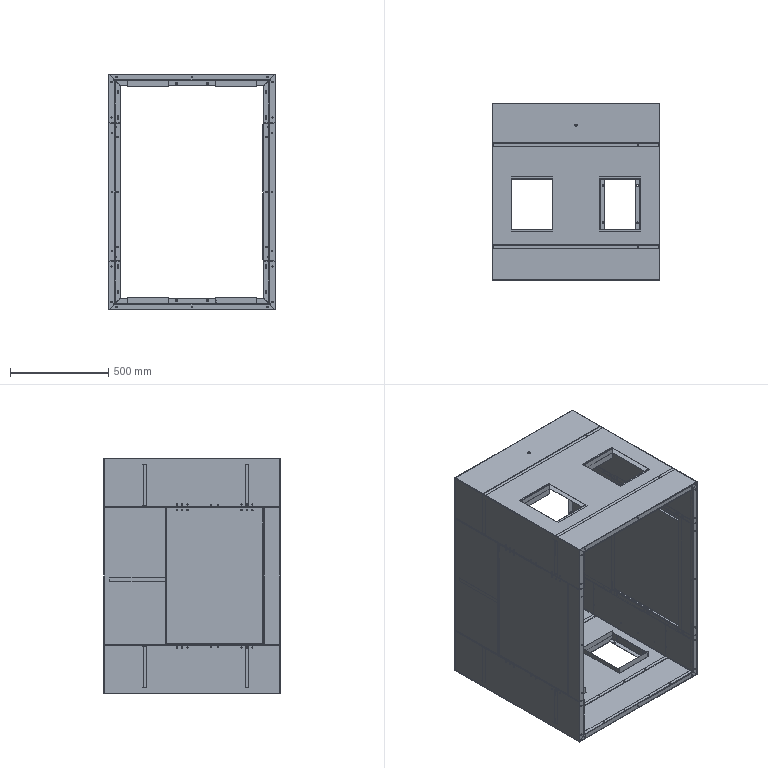Part | SolidWorks | features ReferencePattern 29, MirrorCompFeat 4, LocalLPattern 2, AEMSimFeature 1 | 42 solids | 2382 faces | box 850 x 900 x 1200 mm | volume 10155913 mm3 | plane 1288 | cylinder 982 | spline 112 | commonest cylinder face diameters 5 x188 7 x188 2 x146 4.4 x144 10 x100 8 x58